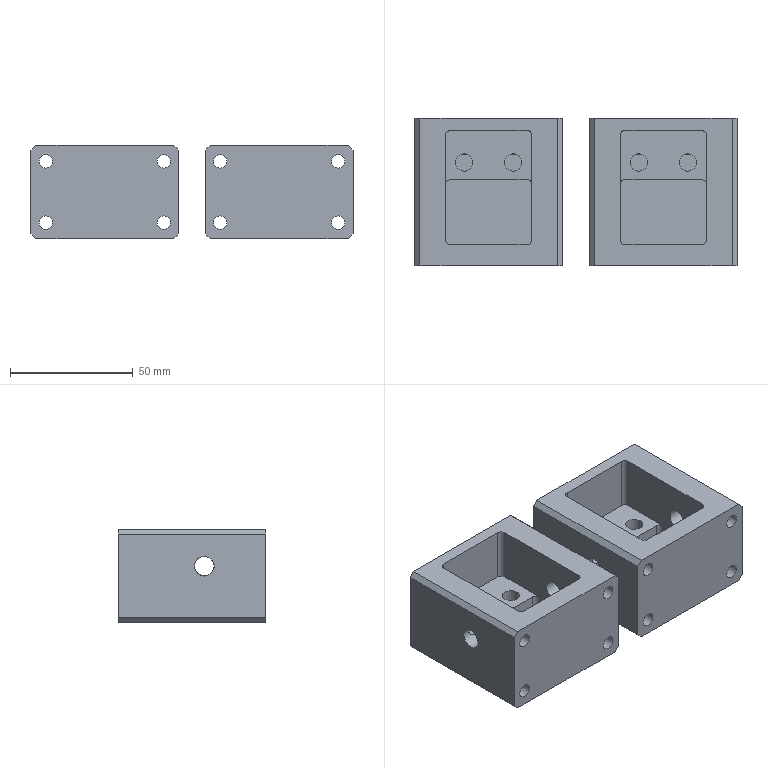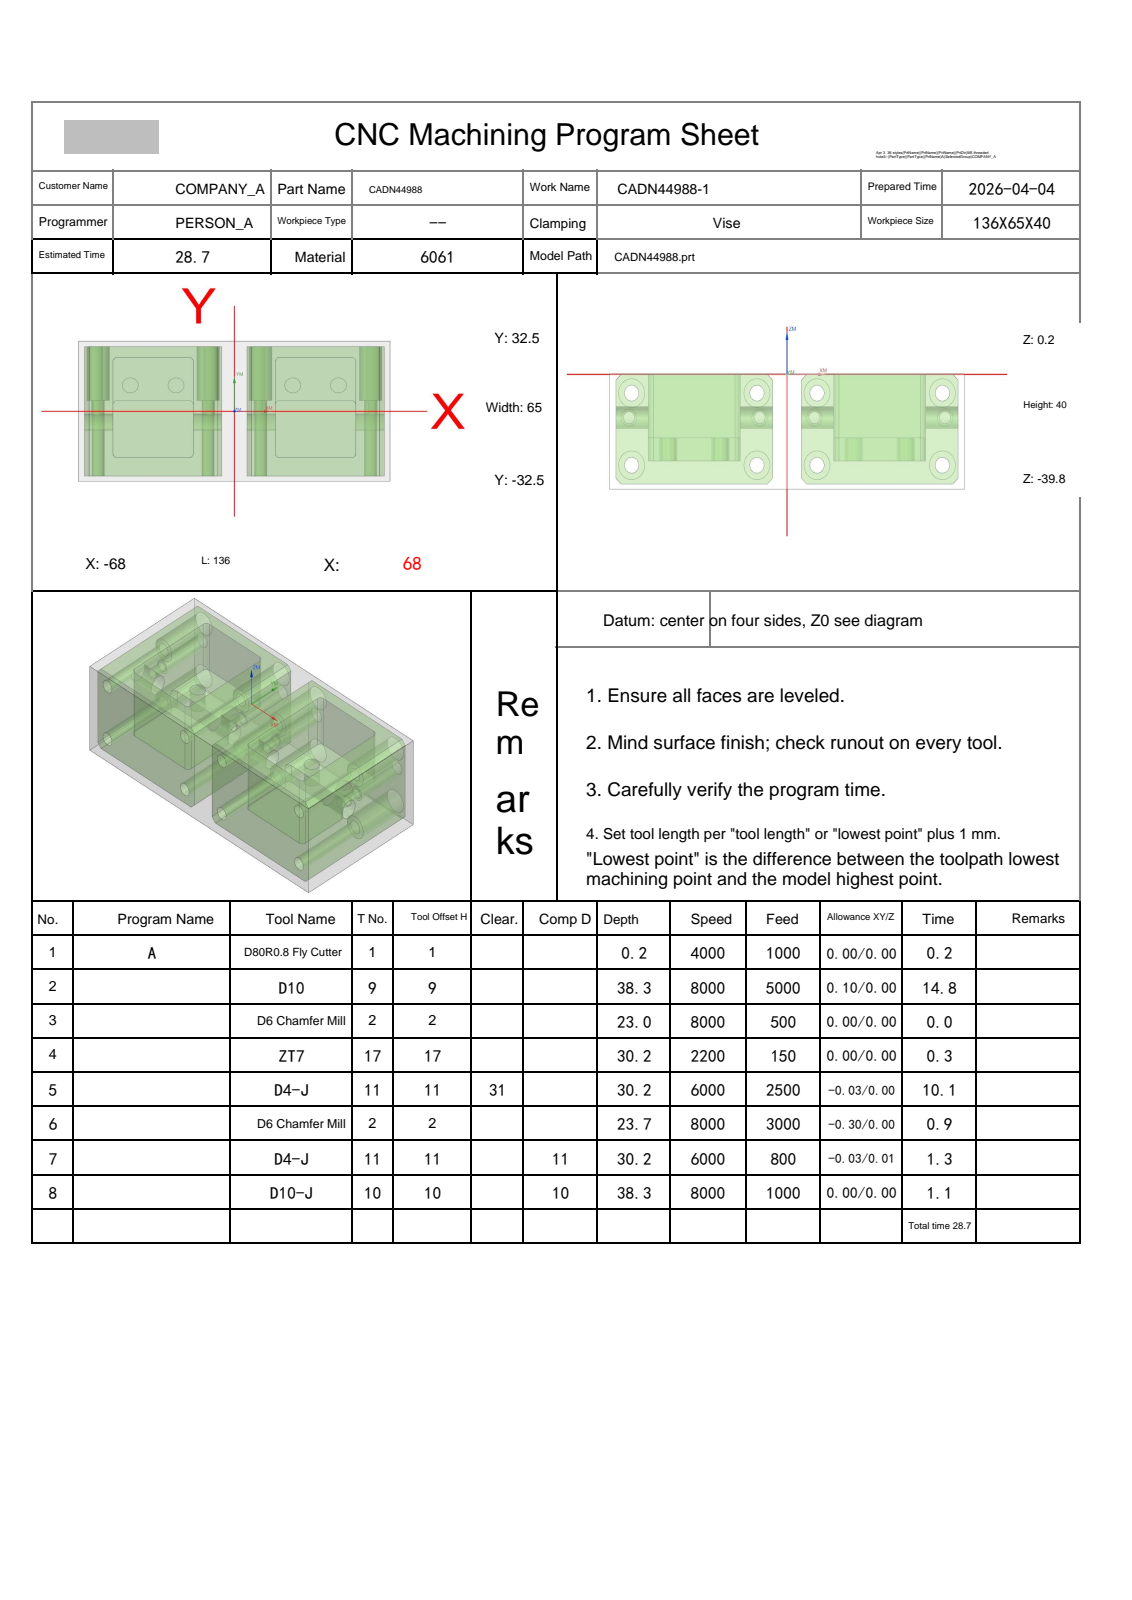NC program | NX | posted by the shop | part box 131 x 60 x 38 mm
Lines 4508 to 4539 of 30516:
N3 T02 M06
(D6 Chamfer Mill  D=6. R=0. H=02 ce=0.00 di=0.00)
G00 G90 G54 X-45.5 Y12. M03 S8000
G43 H02 Z20.
M08
G98 G81 X-45.5 Y12. Z-22.8 R-21. F500.
X-25.5
X25.5
X45.5
G80
G00 Z20.
G91 G28 Z0.0
M05
M09
G91 G28 Z0.0
M01
N4 T17 M06
(ZT7 D=7. DR_a=118 H=17)
G00 G90 G54 X-45.5 Y12. M03 S2200
G43 H17 Z20.
M08
G98 G83 X-45.5 Y12. Z-30. R-21. F150. Q2.
X-25.5
X25.5
X45.5
G80
G00 Z20.
G91 G28 Z0.0
M05
M09
G91 G28 Z0.0
M01